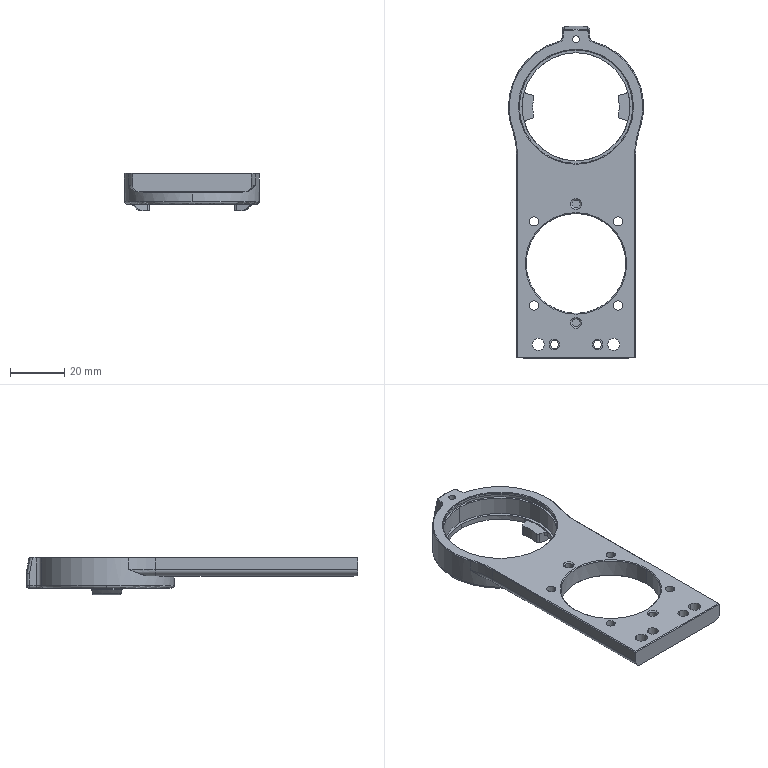NC program | NX | posted with a generic post | part box 50 x 122.9 x 14 mm
Lines 10062 to 10876 of 10876:
(ZLEVEL_PROFILE_COPY_2_COPY , TOOL : D2)
N20044 T17 M6
N20046 G54
N20048 G17 G0 G90 X82.801 Y-15.554 S9500 M3
N20050 G43 Z30. H17
N20052 Z-1.536
N20054 G94 G1 Z-2.536 F1000.
N20056 X82.787 Y-15.904
N20058 G3 X82.881 Y-16.081 R0.2
N20060 X87.123 Y-18.068 R19.
N20062 G1 X87.642 Y-16.133
N20064 G3 X87.59 Y-15.94 R0.2
N20066 G1 X87.364 Y-15.714
N20068 Z-1.536
N20070 G0 X82.801 Y-15.554 Z-1.685
N20072 G1 Z-2.685
N20074 X82.787 Y-15.904
N20076 G3 X82.881 Y-16.081 R0.2
N20078 X87.123 Y-18.068 R19.
N20080 G1 X87.642 Y-16.133
N20082 G3 X87.59 Y-15.94 R0.2
N20084 G1 X87.364 Y-15.714
N20086 Z-1.685
N20088 G0 X82.801 Y-15.554 Z-1.834
N20090 G1 Z-2.834
N20092 X82.787 Y-15.904
N20094 G3 X82.881 Y-16.081 R0.2
N20096 X87.123 Y-18.068 R19.
N20098 G1 X87.642 Y-16.133
N20100 G3 X87.59 Y-15.94 R0.2
N20102 G1 X87.364 Y-15.714
N20104 Z-1.834
N20106 G0 X82.801 Y-15.554 Z-1.983
N20108 G1 Z-2.983
N20110 X82.787 Y-15.904
N20112 G3 X82.881 Y-16.081 R0.2
N20114 X87.123 Y-18.068 R19.
N20116 G1 X87.642 Y-16.133
N20118 G3 X87.59 Y-15.94 R0.2
N20120 G1 X87.364 Y-15.714
N20122 Z-1.983
N20124 G0 X82.801 Y-15.554 Z-2.133
N20126 G1 Z-3.133
N20128 X82.787 Y-15.904
N20130 G3 X82.881 Y-16.081 R0.2
N20132 X87.123 Y-18.068 R19.
N20134 G1 X87.642 Y-16.133
N20136 G3 X87.59 Y-15.94 R0.2
N20138 G1 X87.364 Y-15.714
N20140 Z-2.133
N20142 G0 X82.801 Y-15.554 Z-2.282
N20144 G1 Z-3.282
N20146 X82.787 Y-15.904
N20148 G3 X82.881 Y-16.081 R0.2
N20150 X87.123 Y-18.068 R19.
N20152 G1 X87.642 Y-16.133
N20154 G3 X87.59 Y-15.94 R0.2
N20156 G1 X87.364 Y-15.714
N20158 Z-2.282
N20160 G0 X82.801 Y-15.554 Z-2.431
N20162 G1 Z-3.431
N20164 X82.787 Y-15.904
N20166 G3 X82.881 Y-16.081 R0.2
N20168 X87.123 Y-18.068 R19.
N20170 G1 X87.642 Y-16.133
N20172 G3 X87.59 Y-15.94 R0.2
N20174 G1 X87.364 Y-15.714
N20176 Z-2.431
N20178 G0 X82.801 Y-15.554 Z-2.58
N20180 G1 Z-3.58
N20182 X82.787 Y-15.904
N20184 G3 X82.881 Y-16.081 R0.2
N20186 X87.123 Y-18.068 R19.
N20188 G1 X87.642 Y-16.133
N20190 G3 X87.59 Y-15.94 R0.2
N20192 G1 X87.364 Y-15.714
N20194 Z-2.58
N20196 G0 X82.801 Y-15.554 Z-2.729
N20198 G1 Z-3.729
N20200 X82.787 Y-15.904
N20202 G3 X82.881 Y-16.081 R0.2
N20204 X87.123 Y-18.068 R19.
N20206 G1 X87.642 Y-16.133
N20208 G3 X87.59 Y-15.94 R0.2
N20210 G1 X87.364 Y-15.714
N20212 Z-2.729
N20214 G0 X82.801 Y-15.554 Z-2.878
N20216 G1 Z-3.878
N20218 X82.787 Y-15.904
N20220 G3 X82.881 Y-16.081 R0.2
N20222 X87.123 Y-18.068 R19.
N20224 G1 X87.642 Y-16.133
N20226 G3 X87.59 Y-15.94 R0.2
N20228 G1 X87.364 Y-15.714
N20230 Z-2.878
N20232 G0 X82.802 Y-15.555 Z-3.028
N20234 G1 Z-4.028
N20236 X82.789 Y-15.905
N20238 G3 X82.882 Y-16.082 R0.2
N20240 X87.123 Y-18.068 R19.
N20242 G1 X87.642 Y-16.133
N20244 G3 X87.59 Y-15.94 R0.2
N20246 G1 X87.364 Y-15.714
N20248 Z-3.028
N20250 G0 X82.802 Y-15.555 Z-3.177
N20252 G1 Z-4.177
N20254 X82.789 Y-15.905
N20256 G3 X82.882 Y-16.082 R0.2
N20258 X87.123 Y-18.068 R19.
N20260 G1 X87.642 Y-16.133
N20262 G3 X87.59 Y-15.94 R0.2
N20264 G1 X87.364 Y-15.714
N20266 Z-3.177
N20268 G0 X82.802 Y-15.555 Z-3.326
N20270 G1 Z-4.326
N20272 X82.789 Y-15.905
N20274 G3 X82.882 Y-16.082 R0.2
N20276 X87.123 Y-18.068 R19.
N20278 G1 X87.642 Y-16.133
N20280 G3 X87.59 Y-15.94 R0.2
N20282 G1 X87.364 Y-15.714
N20284 Z-3.326
N20286 G0 X82.802 Y-15.555 Z-3.475
N20288 G1 Z-4.475
N20290 X82.789 Y-15.905
N20292 G3 X82.882 Y-16.082 R0.2
N20294 X87.123 Y-18.068 R19.
N20296 G1 X87.642 Y-16.133
N20298 G3 X87.59 Y-15.94 R0.2
N20300 G1 X87.364 Y-15.714
N20302 Z-3.475
N20304 G0 Z30.
N20306 X98.636
N20308 Z-1.536
N20310 G1 Z-2.536
N20312 X98.41 Y-15.94
N20314 G3 X98.358 Y-16.133 R0.2
N20316 G1 X98.877 Y-18.068
N20318 G3 X103.119 Y-16.081 R19.
N20320 X103.213 Y-15.904 R0.2
N20322 G1 X103.199 Y-15.554
N20324 Z-1.536
N20326 G0 X98.636 Y-15.714 Z-1.685
N20328 G1 Z-2.685
N20330 X98.41 Y-15.94
N20332 G3 X98.358 Y-16.133 R0.2
N20334 G1 X98.877 Y-18.068
N20336 G3 X103.119 Y-16.081 R19.
N20338 X103.213 Y-15.904 R0.2
N20340 G1 X103.199 Y-15.554
N20342 Z-1.685
N20344 G0 X98.636 Y-15.714 Z-1.834
N20346 G1 Z-2.834
N20348 X98.41 Y-15.94
N20350 G3 X98.358 Y-16.133 R0.2
N20352 G1 X98.877 Y-18.068
N20354 G3 X103.119 Y-16.081 R19.
N20356 X103.213 Y-15.904 R0.2
N20358 G1 X103.199 Y-15.554
N20360 Z-1.834
N20362 G0 X98.636 Y-15.714 Z-1.983
N20364 G1 Z-2.983
N20366 X98.41 Y-15.94
N20368 G3 X98.358 Y-16.133 R0.2
N20370 G1 X98.877 Y-18.068
N20372 G3 X103.119 Y-16.081 R19.
N20374 X103.213 Y-15.904 R0.2
N20376 G1 X103.199 Y-15.554
N20378 Z-1.983
N20380 G0 X98.636 Y-15.714 Z-2.133
N20382 G1 Z-3.133
N20384 X98.41 Y-15.94
N20386 G3 X98.358 Y-16.133 R0.2
N20388 G1 X98.877 Y-18.068
N20390 G3 X103.119 Y-16.081 R19.
N20392 X103.213 Y-15.904 R0.2
N20394 G1 X103.199 Y-15.554
N20396 Z-2.133
N20398 G0 X98.636 Y-15.714 Z-2.282
N20400 G1 Z-3.282
N20402 X98.41 Y-15.94
N20404 G3 X98.358 Y-16.133 R0.2
N20406 G1 X98.877 Y-18.068
N20408 G3 X103.119 Y-16.081 R19.
N20410 X103.213 Y-15.904 R0.2
N20412 G1 X103.199 Y-15.554
N20414 Z-2.282
N20416 G0 X98.636 Y-15.714 Z-2.431
N20418 G1 Z-3.431
N20420 X98.41 Y-15.94
N20422 G3 X98.358 Y-16.133 R0.2
N20424 G1 X98.877 Y-18.068
N20426 G3 X103.119 Y-16.081 R19.
N20428 X103.213 Y-15.904 R0.2
N20430 G1 X103.199 Y-15.554
N20432 Z-2.431
N20434 G0 X98.636 Y-15.714 Z-2.58
N20436 G1 Z-3.58
N20438 X98.41 Y-15.94
N20440 G3 X98.358 Y-16.133 R0.2
N20442 G1 X98.877 Y-18.068
N20444 G3 X103.119 Y-16.081 R19.
N20446 X103.213 Y-15.904 R0.2
N20448 G1 X103.199 Y-15.554
N20450 Z-2.58
N20452 G0 X98.636 Y-15.714 Z-2.729
N20454 G1 Z-3.729
N20456 X98.41 Y-15.94
N20458 G3 X98.358 Y-16.133 R0.2
N20460 G1 X98.877 Y-18.068
N20462 G3 X103.119 Y-16.081 R19.
N20464 X103.213 Y-15.904 R0.2
N20466 G1 X103.199 Y-15.554
N20468 Z-2.729
N20470 G0 X98.636 Y-15.714 Z-2.878
N20472 G1 Z-3.878
N20474 X98.41 Y-15.94
N20476 G3 X98.358 Y-16.133 R0.2
N20478 G1 X98.877 Y-18.068
N20480 G3 X103.119 Y-16.081 R19.
N20482 X103.213 Y-15.904 R0.2
N20484 G1 X103.199 Y-15.554
N20486 Z-2.878
N20488 G0 X98.636 Y-15.714 Z-3.028
N20490 G1 Z-4.028
N20492 X98.41 Y-15.94
N20494 G3 X98.358 Y-16.133 R0.2
N20496 G1 X98.877 Y-18.068
N20498 G3 X103.119 Y-16.081 R19.
N20500 X103.213 Y-15.904 R0.2
N20502 G1 X103.199 Y-15.554
N20504 Z-3.028
N20506 G0 X98.636 Y-15.714 Z-3.177
N20508 G1 Z-4.177
N20510 X98.41 Y-15.94
N20512 G3 X98.358 Y-16.133 R0.2
N20514 G1 X98.877 Y-18.068
N20516 G3 X103.119 Y-16.081 R19.
N20518 X103.213 Y-15.904 R0.2
N20520 G1 X103.199 Y-15.554
N20522 Z-3.177
N20524 G0 X98.636 Y-15.714 Z-3.326
N20526 G1 Z-4.326
N20528 X98.41 Y-15.94
N20530 G3 X98.358 Y-16.133 R0.2
N20532 G1 X98.877 Y-18.068
N20534 G3 X103.119 Y-16.081 R19.
N20536 X103.213 Y-15.904 R0.2
N20538 G1 X103.199 Y-15.554
N20540 Z-3.326
N20542 G0 X98.636 Y-15.714 Z-3.475
N20544 G1 Z-4.475
N20546 X98.41 Y-15.94
N20548 G3 X98.358 Y-16.133 R0.2
N20550 G1 X98.877 Y-18.068
N20552 G3 X103.119 Y-16.081 R19.
N20554 X103.213 Y-15.904 R0.2
N20556 G1 X103.199 Y-15.554
N20558 Z-3.475
N20560 G0 Z30.
N20562 Y15.554
N20564 Z-1.536
N20566 G1 Z-2.536
N20568 X103.213 Y15.904
N20570 G3 X103.119 Y16.081 R0.2
N20572 X98.877 Y18.068 R19.
N20574 G1 X98.358 Y16.133
N20576 G3 X98.41 Y15.94 R0.2
N20578 G1 X98.636 Y15.714
N20580 Z-1.536
N20582 G0 X103.199 Y15.554 Z-1.685
N20584 G1 Z-2.685
N20586 X103.213 Y15.904
N20588 G3 X103.119 Y16.081 R0.2
N20590 X98.877 Y18.068 R19.
N20592 G1 X98.358 Y16.133
N20594 G3 X98.41 Y15.94 R0.2
N20596 G1 X98.636 Y15.714
N20598 Z-1.685
N20600 G0 X103.199 Y15.554 Z-1.834
N20602 G1 Z-2.834
N20604 X103.213 Y15.904
N20606 G3 X103.119 Y16.081 R0.2
N20608 X98.877 Y18.068 R19.
N20610 G1 X98.358 Y16.133
N20612 G3 X98.41 Y15.94 R0.2
N20614 G1 X98.636 Y15.714
N20616 Z-1.834
N20618 G0 X103.199 Y15.554 Z-1.983
N20620 G1 Z-2.983
N20622 X103.213 Y15.904
N20624 G3 X103.119 Y16.081 R0.2
N20626 X98.877 Y18.068 R19.
N20628 G1 X98.358 Y16.133
N20630 G3 X98.41 Y15.94 R0.2
N20632 G1 X98.636 Y15.714
N20634 Z-1.983
N20636 G0 X103.199 Y15.554 Z-2.133
N20638 G1 Z-3.133
N20640 X103.213 Y15.904
N20642 G3 X103.119 Y16.081 R0.2
N20644 X98.877 Y18.068 R19.
N20646 G1 X98.358 Y16.133
N20648 G3 X98.41 Y15.94 R0.2
N20650 G1 X98.636 Y15.714
N20652 Z-2.133
N20654 G0 X103.199 Y15.554 Z-2.282
N20656 G1 Z-3.282
N20658 X103.213 Y15.904
N20660 G3 X103.119 Y16.081 R0.2
N20662 X98.877 Y18.068 R19.
N20664 G1 X98.358 Y16.133
N20666 G3 X98.41 Y15.94 R0.2
N20668 G1 X98.636 Y15.714
N20670 Z-2.282
N20672 G0 X103.199 Y15.554 Z-2.431
N20674 G1 Z-3.431
N20676 X103.213 Y15.904
N20678 G3 X103.119 Y16.081 R0.2
N20680 X98.877 Y18.068 R19.
N20682 G1 X98.358 Y16.133
N20684 G3 X98.41 Y15.94 R0.2
N20686 G1 X98.636 Y15.714
N20688 Z-2.431
N20690 G0 X103.199 Y15.554 Z-2.58
N20692 G1 Z-3.58
N20694 X103.213 Y15.904
N20696 G3 X103.119 Y16.081 R0.2
N20698 X98.877 Y18.068 R19.
N20700 G1 X98.358 Y16.133
N20702 G3 X98.41 Y15.94 R0.2
N20704 G1 X98.636 Y15.714
N20706 Z-2.58
N20708 G0 X103.199 Y15.554 Z-2.729
N20710 G1 Z-3.729
N20712 X103.213 Y15.904
N20714 G3 X103.119 Y16.081 R0.2
N20716 X98.877 Y18.068 R19.
N20718 G1 X98.358 Y16.133
N20720 G3 X98.41 Y15.94 R0.2
N20722 G1 X98.636 Y15.714
N20724 Z-2.729
N20726 G0 X103.199 Y15.554 Z-2.878
N20728 G1 Z-3.878
N20730 X103.213 Y15.904
N20732 G3 X103.119 Y16.081 R0.2
N20734 X98.877 Y18.068 R19.
N20736 G1 X98.358 Y16.133
N20738 G3 X98.41 Y15.94 R0.2
N20740 G1 X98.636 Y15.714
N20742 Z-2.878
N20744 G0 X103.199 Y15.554 Z-3.028
N20746 G1 Z-4.028
N20748 X103.213 Y15.904
N20750 G3 X103.119 Y16.081 R0.2
N20752 X98.877 Y18.068 R19.
N20754 G1 X98.358 Y16.133
N20756 G3 X98.41 Y15.94 R0.2
N20758 G1 X98.636 Y15.714
N20760 Z-3.028
N20762 G0 X103.199 Y15.554 Z-3.177
N20764 G1 Z-4.177
N20766 X103.213 Y15.904
N20768 G3 X103.119 Y16.081 R0.2
N20770 X98.877 Y18.068 R19.
N20772 G1 X98.358 Y16.133
N20774 G3 X98.41 Y15.94 R0.2
N20776 G1 X98.636 Y15.714
N20778 Z-3.177
N20780 G0 X103.199 Y15.554 Z-3.326
N20782 G1 Z-4.326
N20784 X103.213 Y15.904
N20786 G3 X103.119 Y16.081 R0.2
N20788 X98.877 Y18.068 R19.
N20790 G1 X98.358 Y16.133
N20792 G3 X98.41 Y15.94 R0.2
N20794 G1 X98.636 Y15.714
N20796 Z-3.326
N20798 G0 X103.199 Y15.554 Z-3.475
N20800 G1 Z-4.475
N20802 X103.213 Y15.904
N20804 G3 X103.119 Y16.081 R0.2
N20806 X98.877 Y18.068 R19.
N20808 G1 X98.358 Y16.133
N20810 G3 X98.41 Y15.94 R0.2
N20812 G1 X98.636 Y15.714
N20814 Z-3.475
N20816 G0 Z30.
N20818 X87.364
N20820 Z-1.536
N20822 G1 Z-2.536
N20824 X87.59 Y15.94
N20826 G3 X87.642 Y16.133 R0.2
N20828 G1 X87.123 Y18.068
N20830 G3 X82.881 Y16.081 R19.
N20832 X82.787 Y15.904 R0.2
N20834 G1 X82.801 Y15.554
N20836 Z-1.536
N20838 G0 X87.364 Y15.714 Z-1.685
N20840 G1 Z-2.685
N20842 X87.59 Y15.94
N20844 G3 X87.642 Y16.133 R0.2
N20846 G1 X87.123 Y18.068
N20848 G3 X82.881 Y16.081 R19.
N20850 X82.787 Y15.904 R0.2
N20852 G1 X82.801 Y15.554
N20854 Z-1.685
N20856 G0 X87.364 Y15.714 Z-1.834
N20858 G1 Z-2.834
N20860 X87.59 Y15.94
N20862 G3 X87.642 Y16.133 R0.2
N20864 G1 X87.123 Y18.068
N20866 G3 X82.881 Y16.081 R19.
N20868 X82.787 Y15.904 R0.2
N20870 G1 X82.801 Y15.554
N20872 Z-1.834
N20874 G0 X87.364 Y15.714 Z-1.983
N20876 G1 Z-2.983
N20878 X87.59 Y15.94
N20880 G3 X87.642 Y16.133 R0.2
N20882 G1 X87.123 Y18.068
N20884 G3 X82.881 Y16.081 R19.
N20886 X82.787 Y15.904 R0.2
N20888 G1 X82.801 Y15.554
N20890 Z-1.983
N20892 G0 X87.364 Y15.714 Z-2.133
N20894 G1 Z-3.133
N20896 X87.59 Y15.94
N20898 G3 X87.642 Y16.133 R0.2
N20900 G1 X87.123 Y18.068
N20902 G3 X82.881 Y16.081 R19.
N20904 X82.787 Y15.904 R0.2
N20906 G1 X82.801 Y15.554
N20908 Z-2.133
N20910 G0 X87.364 Y15.714 Z-2.282
N20912 G1 Z-3.282
N20914 X87.59 Y15.94
N20916 G3 X87.642 Y16.133 R0.2
N20918 G1 X87.123 Y18.068
N20920 G3 X82.881 Y16.081 R19.
N20922 X82.787 Y15.904 R0.2
N20924 G1 X82.801 Y15.554
N20926 Z-2.282
N20928 G0 X87.364 Y15.714 Z-2.431
N20930 G1 Z-3.431
N20932 X87.59 Y15.94
N20934 G3 X87.642 Y16.133 R0.2
N20936 G1 X87.123 Y18.068
N20938 G3 X82.881 Y16.081 R19.
N20940 X82.787 Y15.904 R0.2
N20942 G1 X82.801 Y15.554
N20944 Z-2.431
N20946 G0 X87.364 Y15.714 Z-2.58
N20948 G1 Z-3.58
N20950 X87.59 Y15.94
N20952 G3 X87.642 Y16.133 R0.2
N20954 G1 X87.123 Y18.068
N20956 G3 X82.881 Y16.081 R19.
N20958 X82.787 Y15.904 R0.2
N20960 G1 X82.801 Y15.554
N20962 Z-2.58
N20964 G0 X87.364 Y15.714 Z-2.729
N20966 G1 Z-3.729
N20968 X87.59 Y15.94
N20970 G3 X87.642 Y16.133 R0.2
N20972 G1 X87.123 Y18.068
N20974 G3 X82.881 Y16.081 R19.
N20976 X82.787 Y15.904 R0.2
N20978 G1 X82.801 Y15.554
N20980 Z-2.729
N20982 G0 X87.364 Y15.714 Z-2.878
N20984 G1 Z-3.878
N20986 X87.59 Y15.94
N20988 G3 X87.642 Y16.133 R0.2
N20990 G1 X87.123 Y18.068
N20992 G3 X82.881 Y16.081 R19.
N20994 X82.787 Y15.904 R0.2
N20996 G1 X82.801 Y15.554
N20998 Z-2.878
N21000 G0 X87.364 Y15.714 Z-3.028
N21002 G1 Z-4.028
N21004 X87.59 Y15.94
N21006 G3 X87.642 Y16.133 R0.2
N21008 G1 X87.123 Y18.068
N21010 G3 X82.882 Y16.082 R19.
N21012 X82.789 Y15.905 R0.2
N21014 G1 X82.802 Y15.555
N21016 Z-3.028
N21018 G0 X87.364 Y15.714 Z-3.177
N21020 G1 Z-4.177
N21022 X87.59 Y15.94
N21024 G3 X87.642 Y16.133 R0.2
N21026 G1 X87.123 Y18.068
N21028 G3 X82.882 Y16.082 R19.
N21030 X82.789 Y15.905 R0.2
N21032 G1 X82.802 Y15.555
N21034 Z-3.177
N21036 G0 X87.364 Y15.714 Z-3.326
N21038 G1 Z-4.326
N21040 X87.59 Y15.94
N21042 G3 X87.642 Y16.133 R0.2
N21044 G1 X87.123 Y18.068
N21046 G3 X82.882 Y16.082 R19.
N21048 X82.789 Y15.905 R0.2
N21050 G1 X82.802 Y15.555
N21052 Z-3.326
N21054 G0 X87.364 Y15.714 Z-3.475
N21056 G1 Z-4.475
N21058 X87.59 Y15.94
N21060 G3 X87.642 Y16.133 R0.2
N21062 G1 X87.123 Y18.068
N21064 G3 X82.882 Y16.082 R19.
N21066 X82.789 Y15.905 R0.2
N21068 G1 X82.802 Y15.555
N21070 Z-3.475
N21072 G0 Z30.
N21074 M5
(PLANAR_MILL_1 , TOOL : D6A45)
N21076 T01 M6
N21078 G54
N21080 G17 G0 G90 X18.817 Y-15.981 S9500 M3
N21082 G43 Z30. H1
N21084 Z-6.5
N21086 G94 G1 X18.892 Y-16.108 Z-6.54 F1250.
N21088 X19.229 Y-16.306 Z-6.644
N21090 X19.658 Z-6.759
N21092 X19.995 Y-16.108 Z-6.864
N21094 X20.194 Y-15.771 Z-6.969
N21096 Y-15.342 Z-7.084
N21098 X19.995 Y-15.005 Z-7.189
N21100 X19.658 Y-14.806 Z-7.294
N21102 X19.229 Z-7.408
N21104 X18.892 Y-15.005 Z-7.513
N21106 X18.694 Y-15.342 Z-7.618
N21108 Y-15.771 Z-7.733
N21110 X18.892 Y-16.108 Z-7.838
N21112 X19.229 Y-16.306 Z-7.943
N21114 X19.444 Z-8.
N21116 G3 X20.194 Y-15.556 R0.75
N21118 X19.444 Y-16.306 R-0.75
N21120 X19.877 Y-16.056 R0.5
N21122 G1 Z-6.5
N21124 G0 Z30.
N21126 X3.756 Y-13.475
N21128 Z-6.5
N21130 G1 Z-8.
N21132 X2.95 Y-13.134
N21134 G3 X2.45 Y-14. R1.
N21136 X5. Y-16.55 R2.55
N21138 X2.45 Y-14. R-2.55
N21140 X2.95 Y-14.866 R1.
N21142 G1 X3.756 Y-14.525
N21144 Z-6.5
N21146 G0 Z30.
N21148 X5.542 Y-8.197
N21150 Z-6.5
N21152 G1 X5.55 Y-7.816 Z-6.603
N21154 X5.41 Y-7.59 Z-6.674
N21156 X5.184 Y-7.45 Z-6.745
N21158 X4.816 Z-6.844
N21160 X4.59 Y-7.59 Z-6.915
N21162 X4.45 Y-7.816 Z-6.986
N21164 Y-8.184 Z-7.085
N21166 X4.59 Y-8.41 Z-7.156
N21168 X4.816 Y-8.55 Z-7.227
N21170 X5.184 Z-7.326
N21172 X5.41 Y-8.41 Z-7.397
N21174 X5.55 Y-8.184 Z-7.468
N21176 Y-7.816 Z-7.567
N21178 X5.41 Y-7.59 Z-7.638
N21180 X5.184 Y-7.45 Z-7.71
N21182 X4.816 Z-7.808
N21184 X4.59 Y-7.59 Z-7.879
N21186 X4.45 Y-7.816 Z-7.951
N21188 Y-8. Z-8.
N21190 G3 X5. Y-8.55 R0.55
N21192 X4.45 Y-8. R-0.55
N21194 X4.7 Y-8.433 R0.5
N21196 G1 Z-6.5
N21198 G0 Z30.
N21200 X9.15 Y1.27
N21202 Z-6.5
N21204 G1 Z-8.
N21206 X8.45 Y0.866
N21208 G3 X7.95 Y0. R1.
N21210 G1 Y-4.
N21212 G3 X9. Y-5.05 R1.05
N21214 G2 X11.95 Y-8. R2.95
N21216 G1 Y-16.
N21218 G3 X13. Y-17.05 R1.05
N21220 G1 X13.744
N21222 G3 X14.794 Y-16. R1.05
N21224 G1 Y-15.556
N21226 G2 X16.609 Y-11.87 R4.65
N21228 G3 X16.878 Y-10.511 R1.05
N21230 G2 X16.878 Y10.511 R20.95
N21232 G3 X16.609 Y11.87 R1.05
N21234 G2 X14.794 Y15.556 R4.65
N21236 G1 Y16.
N21238 G3 X13.744 Y17.05 R1.05
N21240 G1 X13.
N21242 G3 X11.95 Y16. R1.05
N21244 G1 Y8.
N21246 G2 X9. Y5.05 R2.95
N21248 G3 X7.95 Y4. R1.05
N21250 G1 Y0.
N21252 G3 X8.45 Y-0.866 R1.
N21254 G1 X9.15 Y-1.27
N21256 Z-6.5
N21258 G0 Z30.
N21260 X5.542 Y7.803
N21262 Z-6.5
N21264 G1 X5.55 Y8.184 Z-6.603
N21266 X5.41 Y8.41 Z-6.674
N21268 X5.184 Y8.55 Z-6.745
N21270 X4.816 Z-6.844
N21272 X4.59 Y8.41 Z-6.915
N21274 X4.45 Y8.184 Z-6.986
N21276 Y7.816 Z-7.085
N21278 X4.59 Y7.59 Z-7.156
N21280 X4.816 Y7.45 Z-7.227
N21282 X5.184 Z-7.326
N21284 X5.41 Y7.59 Z-7.397
N21286 X5.55 Y7.816 Z-7.468
N21288 Y8.184 Z-7.567
N21290 X5.41 Y8.41 Z-7.638
N21292 X5.184 Y8.55 Z-7.71
N21294 X4.816 Z-7.808
N21296 X4.59 Y8.41 Z-7.879
N21298 X4.45 Y8.184 Z-7.951
N21300 Y8. Z-8.
N21302 G3 X5. Y7.45 R0.55
N21304 X4.45 Y8. R-0.55
N21306 X4.7 Y7.567 R0.5
N21308 G1 Z-6.5
N21310 G0 Z30.
N21312 X3.756 Y14.525
N21314 Z-6.5
N21316 G1 Z-8.
N21318 X2.95 Y14.866
N21320 G3 X2.45 Y14. R1.
N21322 X5. Y11.45 R2.55
N21324 X2.45 Y14. R-2.55
N21326 X2.95 Y13.134 R1.
N21328 G1 X3.756 Y13.475
N21330 Z-6.5
N21332 G0 Z30.
N21334 X20.07 Y15.981
N21336 Z-6.5
N21338 G1 X19.995 Y16.108 Z-6.54
N21340 X19.658 Y16.306 Z-6.644
N21342 X19.229 Z-6.759
N21344 X18.892 Y16.108 Z-6.864
N21346 X18.694 Y15.771 Z-6.969
N21348 Y15.342 Z-7.084
N21350 X18.892 Y15.005 Z-7.189
N21352 X19.229 Y14.806 Z-7.294
N21354 X19.658 Z-7.408
N21356 X19.995 Y15.005 Z-7.513
N21358 X20.194 Y15.342 Z-7.618
N21360 Y15.771 Z-7.733
N21362 X19.995 Y16.108 Z-7.838
N21364 X19.658 Y16.306 Z-7.943
N21366 X19.444 Z-8.
N21368 G3 X18.694 Y15.556 R0.75
N21370 X19.444 Y16.306 R-0.75
N21372 X19.011 Y16.056 R0.5
N21374 G1 Z-6.5
N21376 G0 Z30.
N21378 X51.183 Y15.981
N21380 Z-6.5
N21382 G1 X51.108 Y16.108 Z-6.54
N21384 X50.771 Y16.306 Z-6.644
N21386 X50.342 Z-6.759
N21388 X50.005 Y16.108 Z-6.864
N21390 X49.806 Y15.771 Z-6.969
N21392 Y15.342 Z-7.084
N21394 X50.005 Y15.005 Z-7.189
N21396 X50.342 Y14.806 Z-7.294
N21398 X50.771 Z-7.408
N21400 X51.108 Y15.005 Z-7.513
N21402 X51.306 Y15.342 Z-7.618
N21404 Y15.771 Z-7.733
N21406 X51.108 Y16.108 Z-7.838
N21408 X50.771 Y16.306 Z-7.943
N21410 X50.556 Z-8.
N21412 G3 X49.806 Y15.556 R0.75
N21414 X50.556 Y16.306 R-0.75
N21416 X50.123 Y16.056 R0.5
N21418 G1 Z-6.5
N21420 G0 Z30.
N21422 X36.299 Y16.599
N21424 Z-6.5
N21426 G1 Z-8.
N21428 X35.866 Y17.35
N21430 G3 X35. Y17.85 R1.
N21432 X17.15 Y0. R17.85
N21434 X35. Y17.85 R-17.85
N21436 X34.134 Y17.35 R1.
N21438 G1 X33.701 Y16.599
N21440 Z-6.5
N21442 G0 Z30.
N21444 X49.93 Y-15.981
N21446 Z-6.5
N21448 G1 X50.005 Y-16.108 Z-6.54
N21450 X50.342 Y-16.306 Z-6.644
N21452 X50.771 Z-6.759
N21454 X51.108 Y-16.108 Z-6.864
N21456 X51.306 Y-15.771 Z-6.969
N21458 Y-15.342 Z-7.084
N21460 X51.108 Y-15.005 Z-7.189
N21462 X50.771 Y-14.806 Z-7.294
N21464 X50.342 Z-7.408
N21466 X50.005 Y-15.005 Z-7.513
N21468 X49.806 Y-15.342 Z-7.618
N21470 Y-15.771 Z-7.733
N21472 X50.005 Y-16.108 Z-7.838
N21474 X50.342 Y-16.306 Z-7.943
N21476 X50.556 Z-8.
N21478 G3 X51.306 Y-15.556 R0.75
N21480 X50.556 Y-16.306 R-0.75
N21482 X50.989 Y-16.056 R0.5
N21484 G1 Z-6.5
N21486 G0 Z30.
(PLANAR_MILL_1_COPY , TOOL : D6A45)
N21488 X68.476 Y15.85
N21490 Z-6.5
N21492 G1 Z-8.
N21494 X69.866 Y16.668
N21496 G3 X70.79 Y17.05 R1.
N21498 G1 X56.239
N21500 G3 X55.192 Y15.918 R1.05
N21502 G2 X53.391 Y11.87 R4.65
N21504 G3 X53.122 Y10.511 R1.05
N21506 G2 X53.122 Y-10.511 R20.95
N21508 G3 X53.391 Y-11.87 R1.05
N21510 G2 X55.192 Y-15.918 R4.65
N21512 G3 X56.239 Y-17.05 R1.05
N21514 G1 X70.79
N21516 G3 X69.866 Y-16.668 R1.
N21518 G1 X68.476 Y-15.85
N21520 Z-6.5
N21522 G0 Z30.
N21524 X-2.15 Y-20.77
N21526 Z-6.5
N21528 G1 Z-8.
N21530 X-1.45 Y-20.366
N21532 G3 X-0.95 Y-19.5 R1.
N21534 G1 Y19.5
N21536 G3 X-1.45 Y20.366 R1.
N21538 G1 X-2.15 Y20.77
N21540 Z-6.5
N21542 G0 Z30.
(PLANAR_MILL_1_COPY_COPY , TOOL : D6A45)
N21544 X82.509 Y14.442
N21546 Z-2.
N21548 G1 Z-3.5
N21550 X84.057 Y15.989
N21552 G3 X84.316 Y16.955 R1.
N21554 X84.316 Y-16.955 R19.05
N21556 X84.057 Y-15.989 R1.
N21558 G1 X82.509 Y-14.442
N21560 Z-2.
N21562 G0 Z30.
N21564 X103.491
N21566 Z-2.
N21568 G1 Z-3.5
N21570 X101.943 Y-15.989
N21572 G3 X101.684 Y-16.955 R1.
N21574 X101.684 Y16.955 R19.05
N21576 X101.943 Y15.989 R1.
N21578 G1 X103.491 Y14.442
N21580 Z-2.
N21582 G0 Z30.
(PLANAR_MILL_1_COPY_COPY_COPY , TOOL : D6A45)
N21584 X100.367 Y19.189
N21586 Z0.5
N21588 G1 Z-1.
N21590 X99.587 Y18.98
N21592 G3 X98.88 Y18.272 R1.
N21594 G1 X98.31 Y16.146
N21596 G2 X96.033 Y14.741 R1.95
N21598 G3 X89.967 Y14.741 R15.05
N21600 G2 X87.69 Y16.146 R1.95
N21602 G1 X87.12 Y18.272
N21604 G3 X86.413 Y18.98 R1.
N21606 G1 X85.633 Y19.189
N21608 Z0.5
N21610 G0 Z30.
N21612 Y-19.189
N21614 Z0.5
N21616 G1 Z-1.
N21618 X86.413 Y-18.98
N21620 G3 X87.12 Y-18.272 R1.
N21622 G1 X87.69 Y-16.146
N21624 G2 X89.967 Y-14.741 R1.95
N21626 G3 X96.033 Y-14.741 R15.05
N21628 G2 X98.31 Y-16.146 R1.95
N21630 G1 X98.88 Y-18.272
N21632 G3 X99.587 Y-18.98 R1.
N21634 G1 X100.367 Y-19.189
N21636 Z0.5
N21638 G0 Z30.
N21640 M5
N21642 M2